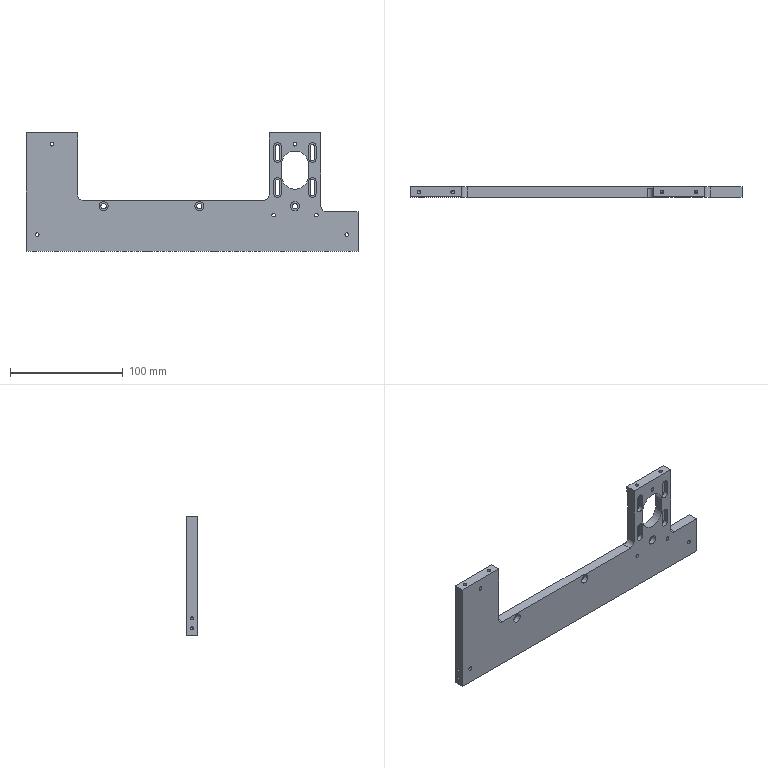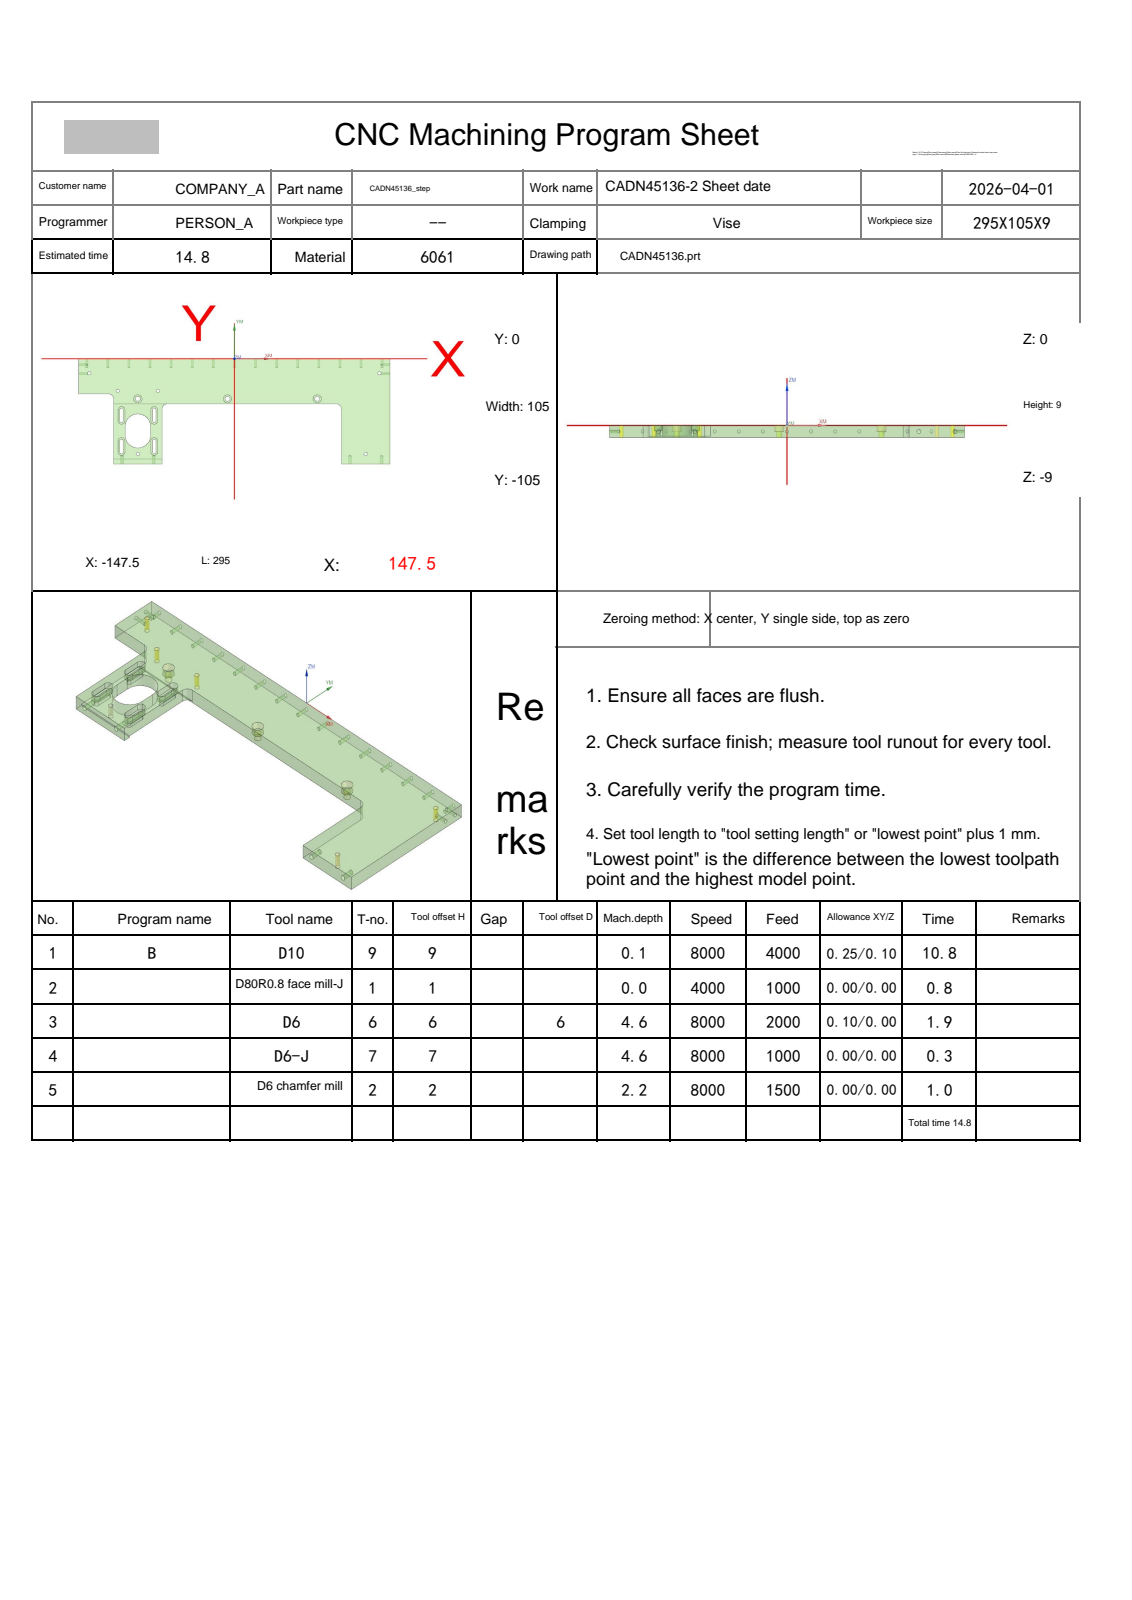NC program | NX | posted by the shop | part box 295 x 9 x 105 mm
Lines 1 to 770 of 3343:
%
O0001
(Machine time: 15.76 MIN)
(===Total Tool:5===)
(T9=D10     D=10.  R=0.   D-  H09 Z=0.1   )
(T1=D80R0.8 face mill-J D=80.  R=0.8  D-  H01 Z=0.    )
(T6=D6      D=6.   R=0.   D6  H06 Z=-4.6  )
(T7=D6-J    D=6.   R=0.   D7  H07 Z=-4.6  )
(T2=D6 chamfer mill   D=6.   R=0.   D-  H02 Z=-2.2  )
G80 G90 G17 G49 G40
G91 G28 Z0
M01
N1 T09 M06
(D10  D=10. R=0. H=09 ce=0.25 di=0.10)
G00 G90 G54 X-1.042 Y13.599 M03 S8000
G43 H09 Z20.
M08
Z2.1
G01 X-1.024 Y13.501 Z1.476 F4000.
X-1.006 Y13.402 Z1.228
X-.988 Y13.304 Z1.046
X-.97 Y13.206 Z.9
X-.952 Y13.107 Z.777
X-.934 Y13.009 Z.672
X-.916 Y12.911 Z.58
X-.898 Y12.812 Z.5
X-.88 Y12.714 Z.43
X-.862 Y12.616 Z.368
X-.844 Y12.517 Z.314
X-.826 Y12.419 Z.267
X-.808 Y12.32 Z.227
X-.79 Y12.222 Z.192
X-.772 Y12.124 Z.164
X-.754 Y12.025 Z.14
X-.737 Y11.927 Z.123
X-.719 Y11.829 Z.11
X-.701 Y11.73 Z.103
X-.683 Y11.632 Z.1
X-.271 Y9.38
G03 X.02 Y9.01 I.503 J.096
X3.263 Y8.4 I3.513 J9.761
X11.624 Y8.192 I8.361 J167.742
X13.491 Y8.202 I0.0 J167.951
G01 X148.128 Y8.183
G02 X154.101 Y4.173 I-.143 J-6.666
X155.462 Y-1.639 I-15.018 J-6.584
X155.704 Y-9.746 I-136.186 J-8.107
X155.695 Y-11.233 I-136.427 J0.0
G01 X155.683 Y-105.63
G02 X151.671 Y-111.602 I-6.664 J.143
X145.703 Y-112.976 I-6.659 J15.278
X136.222 Y-113.219 I-9.481 J184.401
X133.468 Y-113.199 I0.0 J184.644
G01 X-148.17 Y-113.181
G02 X-153.997 Y-109.369 I.158 J6.6
X-155.442 Y-103.579 I14.146 J6.608
X-155.706 Y-95.369 I127.878 J8.21
X-155.695 Y-93.745 I128.141 J0.0
G01 X-155.68 Y.671
G02 X-151.811 Y6.525 I6.619 J-.169
X-145.861 Y7.962 I6.676 J-14.612
X-137.748 Y8.204 I8.112 J-135.802
X-136.266 Y8.196 I0.0 J-136.044
G01 X-2.686 Y8.179
G03 X4.722 Y7.563 I23.47 J237.591
X15.046 Y7.398 I10.324 J322.404
X16.288 Y7.4 I0.0 J322.569
G01 X146.108 Y7.384
G02 X152.709 Y3.222 I-.293 J-7.781
X154.521 Y-3.04 I-14.437 J-7.57
X154.905 Y-11.965 I-103.523 J-8.925
X154.892 Y-13.589 I-103.907 J0.0
G01 X154.879 Y-103.707
G02 X150.784 Y-110.174 I-7.756 J.381
X144.376 Y-112.031 I-7.651 J14.414
X135.464 Y-112.405 I-8.912 J105.999
X133.827 Y-112.392 I0.0 J106.373
G01 X-146.167 Y-112.381
G02 X-152.66 Y-108.304 I.342 J7.752
X-154.529 Y-101.89 I14.346 J7.66
X-154.906 Y-92.925 I106.524 J8.965
X-154.893 Y-91.261 I106.901 J0.0
G01 X-154.881 Y-1.333
G02 X-150.852 Y5.129 I7.744 J-.341
X-144.767 Y6.983 I7.517 J-13.763
X-136.458 Y7.391 I8.309 J-84.332
X-135.421 Y7.385 I0.0 J-84.741
G01 X-4.322 Y7.377
G02 X3.942 Y6.829 I-44.818 J-737.899
G03 X16.194 Y6.592 I12.252 J316.992
X18.528 Y6.601 I0.0 J317.229
G01 X144.268 Y6.579
G02 X151.862 Y1.656 I-.345 J-8.85
X153.721 Y-5.172 I-16.699 J-8.211
X154.102 Y-14.54 I-114.771 J-9.369
X154.091 Y-16.121 I-115.153 J0.0
G01 X154.078 Y-101.781
G02 X149.123 Y-109.38 I-8.847 J.353
X142.283 Y-111.226 I-8.208 J16.824
X133.353 Y-111.594 I-8.931 J108.095
X132.214 Y-111.588 I0.0 J108.463
G01 X-144.326 Y-111.576
G02 X-151.833 Y-106.709 I.392 J8.829
X-153.687 Y-100.123 I16.208 J8.116
X-154.097 Y-90.987 I101.659 J9.136
X-154.088 Y-89.656 I102.068 J0.0
G01 X-154.083 Y-3.356
G02 X-149.226 Y4.322 I8.844 J-.219
X-142.488 Y6.202 I8.189 J-16.333
X-133.467 Y6.595 I9.02 J-103.367
X-132.26 Y6.588 I0.0 J-103.76
G01 X-5.88 Y6.582
G02 X4.55 Y6.018 I-22.742 J-517.372
G03 X18.104 Y5.791 I13.554 J404.888
X20.929 Y5.801 I0.0 J405.115
G01 X142.428 Y5.779
G02 X150.985 Y.337 I-.13 J-9.652
X152.881 Y-6.654 I-17.825 J-8.587
X153.298 Y-16.352 I-112.524 J-9.698
X153.289 Y-17.842 I-112.941 J0.0
G01 X153.278 Y-99.901
G02 X147.729 Y-108.54 I-9.678 J.115
X140.572 Y-110.412 I-8.649 J18.457
X130.965 Y-110.798 I-9.607 J119.204
X129.543 Y-110.79 I0.0 J119.59
G01 X-142.357 Y-110.78
G02 X-151.013 Y-105.281 I.07 J9.672
X-152.897 Y-98.204 I18.157 J8.623
X-153.299 Y-88.521 I116.384 J9.683
X-153.289 Y-87.016 I116.787 J0.0
G01 X-153.279 Y-5.116
G02 X-147.731 Y3.538 I9.686 J-.104
X-140.49 Y5.42 I8.693 J-18.576
X-130.936 Y5.798 I9.553 J-120.599
X-129.54 Y5.79 I0.0 J-120.977
G01 X-6.76 Y5.776
G02 X5.245 Y5.203 I-27.413 J-700.319
G03 X19.831 Y4.991 I14.586 J501.673
X23.008 Y5.001 I0.0 J501.885
G01 X140.748 Y4.978
X140.781
G02 X150.278 Y-1.205 I0.0 J-10.385
X152.099 Y-8.47 I-20.118 J-8.901
X152.494 Y-18.28 I-121.393 J-9.81
X152.487 Y-19.579 I-121.789 J0.0
G01 X152.477 Y-98.199
X152.478 Y-98.282
G02 X146.307 Y-107.772 I-10.383 J0.0
X138.891 Y-109.614 I-8.969 J20.269
X129.14 Y-109.994 I-9.751 J124.677
X127.861 Y-109.988 I0.0 J125.057
G01 X-140.758 Y-109.975
X-140.792
G02 X-150.243 Y-103.866 I0.0 J10.365
X-152.115 Y-96.374 I20.166 J9.018
X-152.494 Y-86.658 I124.333 J9.716
X-152.488 Y-85.424 I124.712 J0.0
G01 X-152.474 Y-6.724
Y-6.712
G02 X-146.318 Y2.767 I10.375 J0.0
X-139.141 Y4.587 I8.872 J-19.921
X-129.221 Y4.996 I9.92 J-119.985
X-127.792 Y4.988 I0.0 J-120.395
G01 X-7.652 Y4.975
G02 X5.16 Y4.417 I-21.37 J-638.689
G03 X20.407 Y4.192 I15.247 J516.842
X23.488 Y4.202 I0.0 J517.067
G01 X139.148 Y4.177
X139.271 Y4.178
G02 X145.984 Y1.999 I0.0 J-11.431
X150.263 Y-4.534 I-8.054 J-9.944
X151.499 Y-12.66 I-32.537 J-9.105
X151.719 Y-25.287 I-362.488 J-12.627
X151.698 Y-29.217 I-362.708 J0.0
G01 X151.677 Y-96.557
X151.679 Y-96.726
G02 X149.706 Y-103.204 I-11.62 J0.0
X143.206 Y-107.687 I-10.008 J7.557
X135.249 Y-108.976 I-9.062 J30.727
X124.188 Y-109.209 I-11.061 J262.82
X121.653 Y-109.197 I0.0 J263.052
G01 X-139.127 Y-109.175
X-139.258 Y-109.176
G02 X-145.952 Y-107.022 I0.0 J11.48
X-150.277 Y-100.42 I8.041 J9.985
X-151.506 Y-92.212 I32.969 J9.136
X-151.718 Y-79.639 I373.131 J12.573
X-151.698 Y-75.735 I373.343 J0.0
G01 X-151.673 Y-8.315
Y-8.213
G02 X-149.486 Y-1.503 I11.387 J0.0
X-142.871 Y2.792 I9.977 J-8.126
X-134.74 Y4.005 I9.092 J-33.074
X-122.127 Y4.219 I12.613 J-371.929
X-118.182 Y4.198 I0.0 J-372.143
G01 X-8.522 Y4.174
G02 X5.864 Y3.601 I-23.554 J-772.256
G03 X21.43 Y3.394 I15.566 J585.251
X24.368 Y3.402 I0.0 J585.458
G01 X137.468 Y3.382
G02 X137.692 Y3.384 I.224 J-13.158
X143.714 Y1.926 I0.0 J-13.16
X149.031 Y-4.551 I-6.152 J-10.472
X150.617 Y-12.853 I-27.515 J-9.559
X150.914 Y-24.635 I-233.501 J-11.782
X150.896 Y-27.568 I-233.798 J0.0
G01 X150.878 Y-94.988
G02 X150.88 Y-95.199 I-13.158 J-.211
X149.452 Y-101.161 I-13.159 J0.0
X143.124 Y-106.463 I-10.434 J6.026
X135.236 Y-108.073 I-9.392 J25.881
X124.51 Y-108.403 I-10.725 J174.014
X122.603 Y-108.393 I0.0 J174.344
G01 X-137.537 Y-108.377
X-137.735 Y-108.378
G02 X-143.913 Y-106.81 I0.0 J12.949
X-149.074 Y-100.334 I6.443 J10.429
X-150.615 Y-92.187 I27.721 J9.461
X-150.915 Y-80.371 I232.213 J11.816
X-150.896 Y-77.392 I232.513 J0.0
G01 X-150.877 Y-9.972
X-150.878 Y-9.775
G02 X-149.352 Y-3.662 I13. J0.0
X-143.008 Y1.506 I10.402 J-6.291
X-134.874 Y3.101 I9.476 J-26.788
X-124.315 Y3.401 I10.559 J-185.945
X-122.56 Y3.392 I0.0 J-186.244
G01 X-9.38 Y3.375
G02 X5.387 Y2.825 I-16.941 J-653.015
G03 X22.135 Y2.593 I16.748 J603.489
X25.488 Y2.602 I0.0 J603.721
G01 X136.188 Y2.577
X136.37 Y2.579
G02 X142.462 Y1.185 I0.0 J-14.012
X148.057 Y-5.299 I-5.926 J-10.769
X149.766 Y-13.571 I-26.358 J-9.757
X150.109 Y-25.105 I-193.559 J-11.534
X150.094 Y-27.564 I-193.902 J0.0
G01 X150.079 Y-93.464
G02 X150.082 Y-93.753 I-14.601 J-.289
X148.823 Y-99.686 I-14.604 J0.0
X142.273 Y-105.528 I-10.848 J5.57
X134.325 Y-107.233 I-9.618 J25.454
X123.377 Y-107.601 I-10.948 J162.529
X121.533 Y-107.591 I0.0 J162.898
G01 X-135.967 Y-107.579
G02 X-136.251 Y-107.582 I-.285 J14.603
X-142.189 Y-106.321 I0.0 J14.605
X-148.007 Y-99.82 I5.558 J10.827
X-149.756 Y-91.556 I25.794 J9.774
X-150.099 Y-80.759 I169.356 J10.797
X-150.09 Y-79.004 I169.7 J0.0
G01 X-150.074 Y-11.344
G02 X-150.076 Y-11.137 I14.003 J.207
X-148.625 Y-4.929 I14.004 J0.0
X-142.165 Y.57 I10.742 J-6.074
X-134.046 Y2.256 I9.668 J-26.161
X-122.365 Y2.611 I11.681 J-192.34
X-119.813 Y2.594 I0.0 J-192.695
G01 X-10.233 Y2.577
G02 X6.173 Y2.006 I-18.598 J-770.274
G03 X22.893 Y1.796 I16.72 J665.43
X25.888 Y1.802 I0.0 J665.64
G01 X134.588 Y1.783
G02 X134.896 Y1.786 I.308 J-15.827
X140.912 Y.598 I0.0 J-15.83
X147.098 Y-6.055 I-5.326 J-11.154
X148.894 Y-14.065 I-25.062 J-9.825
X149.298 Y-25.195 I-153.026 J-11.13
X149.289 Y-26.934 I-153.43 J0.0
G01 X149.276 Y-92.194
G02 X149.278 Y-92.466 I-15.489 J-.271
X148.051 Y-98.508 I-15.491 J0.0
X141.479 Y-104.583 I-11.107 J5.424
X133.155 Y-106.42 I-9.985 J25.465
X121.693 Y-106.805 I-11.462 J170.608
X119.564 Y-106.791 I0.0 J170.992
G01 X-134.736 Y-106.775
G02 X-134.974 Y-106.777 I-.239 J15.483
X-140.982 Y-105.564 I0.0 J15.484
X-147.132 Y-98.864 I5.426 J11.153
X-148.903 Y-90.843 I25.455 J9.827
X-149.299 Y-79.739 I155.791 J11.104
X-149.289 Y-77.972 I156.186 J0.0
G01 X-149.271 Y-12.633
X-149.272 Y-12.451
G02 X-147.976 Y-6.335 I15.078 J0.0
X-141.234 Y-.315 I11.137 J-5.687
X-132.81 Y1.45 I9.979 J-26.643
X-121.588 Y1.802 I11.222 J-178.732
X-119.618 Y1.791 I0.0 J-179.084
G01 X-11.158 Y1.779
G02 X5.854 Y1.221 I-14.287 J-695.118
G03 X22.663 Y1. I16.809 J638.744
X24.689 Y1.003 I0.0 J638.965
G01 X133.388 Y.98
G02 X133.653 Y.982 I.265 J-16.768
X139.651 Y-.128 I0.0 J-16.77
X146.18 Y-6.878 I-5.078 J-11.443
X148.09 Y-15.268 I-25.295 J-10.171
X148.502 Y-26.848 I-162.533 J-11.581
X148.489 Y-28.858 I-162.946 J0.0
G01 X148.472 Y-90.997
G02 X148.474 Y-91.236 I-16.272 J-.238
X147.26 Y-97.402 I-16.274 J0.0
X140.574 Y-103.699 I-11.368 J5.371
X132.336 Y-105.58 I-10.09 J25.217
X121.468 Y-105.99 I-10.867 J143.791
X120.186 Y-105.984 I0.0 J144.201
G01 X-133.474 Y-105.973
G02 X-133.725 Y-105.974 I-.251 J16.335
X-139.877 Y-104.772 I0.0 J16.337
X-146.157 Y-98.172 I5.319 J11.349
X-148.062 Y-90.024 I24.703 J10.071
X-148.491 Y-79.056 I139.98 J10.968
X-148.484 Y-77.715 I140.409 J0.0
G01 X-148.473 Y-14.056
G02 X-148.475 Y-13.804 I16.505 J.251
X-147.314 Y-7.724 I16.507 J0.0
X-140.649 Y-1.334 I11.387 J-5.208
X-132.343 Y.579 I10.135 J-25.013
X-121.513 Y.989 I10.829 J-142.782
X-120.273 Y.984 I0.0 J-143.192
G01 X-11.173 Y.972
G02 X6.881 Y.395 I-21.697 J-962.456
G03 X23.793 Y.2 I16.912 J730.973
X25.969 Y.203 I0.0 J731.169
G01 X132.028 Y.182
G02 X132.357 Y.185 I.329 J-18.071
X138.464 Y-.878 I0.0 J-18.074
X145.286 Y-7.734 I-4.904 J-11.7
X147.262 Y-16.192 I-25.181 J-10.344
X147.701 Y-27.987 I-158.212 J-11.794
X147.688 Y-30.021 I-158.651 J0.0
G01 X147.672 Y-89.681
G02 X147.674 Y-89.962 I-17.445 J-.281
X146.529 Y-96.18 I-17.447 J0.0
X139.81 Y-102.765 I-11.615 J5.131
X131.754 Y-104.717 I-10.17 J24.374
X120.47 Y-105.19 I-11.284 J134.156
X119.048 Y-105.183 I0.0 J134.63
G01 X-132.212 Y-105.172
G02 X-132.475 Y-105.174 I-.263 J17.377
X-138.709 Y-104.017 I0.0 J17.379
X-145.341 Y-97.139 I5.196 J11.647
X-147.276 Y-88.669 I25.668 J10.318
X-147.702 Y-76.836 I163.921 J11.832
X-147.689 Y-74.759 I164.347 J0.0
G01 X-147.673 Y-15.339
G02 X-147.675 Y-15.055 I17.541 J.284
X-146.536 Y-8.838 I17.543 J0.0
X-139.664 Y-2.171 I11.662 J-5.146
X-131.438 Y-.251 I10.223 J-25.219
X-120.35 Y.188 I11.087 J-139.656
X-119.05 Y.182 I0.0 J-140.096
G01 X-12.03 Y.174
G02 X6.245 Y-.382 I-15.656 J-814.736
G03 X23.967 Y-.6 I17.722 J718.369
X26.289 Y-.597 I0.0 J718.587
G01 X130.748 Y-.618
G02 X131.097 Y-.615 I.348 J-19.457
X137.203 Y-1.598 I0.0 J-19.46
X144.348 Y-8.47 I-4.602 J-11.933
X146.408 Y-16.829 I-24.414 J-10.451
X146.885 Y-28.059 I-131.929 J-11.23
X146.879 Y-29.295 I-132.406 J0.0
G01 X146.875 Y-88.315
G02 X146.878 Y-88.657 I-19.049 J-.342
X145.846 Y-94.84 I-19.052 J0.0
X138.847 Y-101.929 I-11.926 J4.775
X130.633 Y-103.912 I-10.35 J24.864
X119.202 Y-104.39 I-11.431 J136.647
X117.767 Y-104.382 I0.0 J137.125
G01 X-130.853 Y-104.374
G02 X-131.167 Y-104.377 I-.314 J19.039
X-137.301 Y-103.361 I0.0 J19.042
X-144.41 Y-96.392 I4.731 J11.936
X-146.423 Y-88.028 I24.936 J10.426
X-146.888 Y-76.687 I137.999 J11.341
X-146.882 Y-75.321 I138.464 J0.0
G01 X-146.875 Y-16.701
G02 X-146.878 Y-16.368 I19.259 J.333
X-145.88 Y-10.25 I19.262 J0.0
X-138.893 Y-3.092 I11.947 J-4.672
X-130.764 Y-1.103 I10.314 J-24.541
X-119.319 Y-.612 I11.445 J-133.096
X-117.898 Y-.619 I0.0 J-133.587
G01 X-12.878 Y-.624
G02 X6.085 Y-1.173 I-13.148 J-780.897
G03 X24.808 Y-1.403 I18.723 J763.395
X27.889 Y-1.397 I0.0 J763.625
G01 X129.708 Y-1.422
G02 X130.007 Y-1.419 I.298 J-19.874
X136.24 Y-2.422 I0.0 J-19.876
X143.541 Y-9.474 I-4.665 J-12.135
X145.603 Y-17.914 I-24.987 J-10.575
X146.084 Y-29.282 I-134.004 J-11.368
X146.079 Y-30.46 I-134.485 J0.0
G01 X146.074 Y-87.08
G02 X146.077 Y-87.434 I-20.386 J-.354
X145.117 Y-93.62 I-20.389 J0.0
X138.173 Y-100.971 I-12.128 J4.501
X129.754 Y-103.085 I-10.592 J24.363
X118.099 Y-103.589 I-11.655 J134.466
X116.649 Y-103.581 I0.0 J134.971
G01 X-129.731 Y-103.571
G02 X-130.037 Y-103.574 I-.306 J19.668
X-136.337 Y-102.538 I0.0 J19.67
X-143.588 Y-95.42 I4.798 J12.14
X-145.63 Y-86.816 I25.615 J10.625
X-146.086 Y-75.438 I141.783 J11.378
X-146.081 Y-74.188 I142.239 J0.0
G01 X-146.074 Y-17.888
G02 X-146.076 Y-17.563 I20.449 J.325
X-145.133 Y-11.425 I20.452 J0.0
X-138.05 Y-3.972 I12.182 J-4.486
X-129.535 Y-1.892 I10.609 J-24.965
X-118.038 Y-1.413 I11.497 J-137.63
X-116.668 Y-1.42 I0.0 J-138.109
G01 X-12.848 Y-1.429
G02 X6.717 Y-1.988 I-16.701 J-927.382
G03 X25.212 Y-2.202 I18.496 J797.81
X28.289 Y-2.196 I0.0 J798.024
G01 X128.108 Y-2.214
G02 X128.579 Y-2.209 I.47 J-22.807
X134.75 Y-3.059 I0.0 J-22.812
X142.62 Y-10.214 I-4.101 J-12.418
X144.778 Y-18.789 I-24.668 J-10.765
X145.284 Y-30.396 I-132.82 J-11.607
X145.278 Y-31.654 I-133.326 J0.0
G01 X145.279 Y-85.634
G02 X145.284 Y-86.096 I-22.726 J-.462
X144.428 Y-92.274 I-22.731 J0.0
X137.082 Y-100.213 I-12.469 J4.169
X128.491 Y-102.301 I-10.72 J25.386
X116.831 Y-102.787 I-11.66 J139.7
X115.465 Y-102.78 I0.0 J140.186
G01 X-128.195 Y-102.778
G02 X-128.635 Y-102.782 I-.44 J22.458
X-134.832 Y-101.91 I0.0 J22.463
X-142.567 Y-94.895 I4.168 J12.367
X-144.737 Y-86.57 I23.91 J10.679
X-145.28 Y-75.018 I122.634 J11.553
X-145.275 Y-73.868 I123.177 J0.0
G01 X-145.279 Y-19.408
G02 X-145.284 Y-18.95 I23.289 J.458
X-144.489 Y-12.918 I23.293 J0.0
X-137.252 Y-4.865 I12.466 J-3.925
X-128.831 Y-2.736 I10.685 J-24.542
X-117.395 Y-2.221 I11.436 J-126.686
X-116.367 Y-2.225 I0.0 J-127.201
G01 X-13.507 Y-2.228
G02 X6.953 Y-2.791 I-15.92 J-950.714
G03 X25.301 Y-3.001 I18.348 J800.206
X28.289 Y-2.996 I0.0 J800.416
G01 X127.309 Y-3.02
G02 X127.645 Y-3.018 I.336 J-22.38
X133.941 Y-3.922 I0.0 J-22.382
X141.858 Y-11.279 I-4.313 J-12.579
X143.969 Y-19.79 I-25.303 J-10.791
X144.484 Y-31.582 I-134.68 J-11.792
X144.478 Y-32.895 I-135.195 J0.0
G01 X144.474 Y-84.715
G02 X144.477 Y-85.112 I-22.579 J-.397
X143.576 Y-91.429 I-22.582 J0.0
X136.33 Y-99.306 I-12.56 J4.284
X127.67 Y-101.473 I-10.878 J25.079
X115.643 Y-101.989 I-12.027 J139.765
X114.085 Y-101.981 I0.0 J140.281
G01 X-127.015 Y-101.978
G02 X-127.483 Y-101.982 I-.468 J23.641
X-133.738 Y-101.14 I0.0 J23.645
X-141.795 Y-93.853 I4.078 J12.605
X-143.943 Y-85.436 I24.626 J10.769
X-144.481 Y-73.721 I127.363 J11.715
X-144.475 Y-72.492 I127.901 J0.0
G01 X-144.478 Y-20.513
G02 X-144.482 Y-20.07 I24.308 J.442
X-143.716 Y-14.018 I24.312 J0.0
X-136.256 Y-5.66 I12.7 J-3.827
X-127.674 Y-3.528 I10.832 J-25.269
X-115.667 Y-3.011 I12.008 J-139.276
X-114.089 Y-3.02 I0.0 J-139.792
G01 X-14.349 Y-3.026
G02 X7.031 Y-3.59 I-14.475 J-953.625
G03 X25.408 Y-3.801 I18.377 J802.198
X28.289 Y-3.795 I0.0 J802.408
G01 X125.948 Y-3.816
G02 X126.362 Y-3.812 I.414 J-24.772
X132.6 Y-4.61 I0.0 J-24.775
X140.999 Y-12.12 I-3.91 J-12.826
X143.161 Y-20.782 I-25.409 J-10.943
X143.683 Y-32.699 I-135.681 J-11.917
X143.677 Y-34.046 I-136.204 J0.0
G01 Y-83.386
G02 X143.682 Y-83.862 I-24.664 J-.475
X142.855 Y-90.194 I-24.668 J0.0
X135.55 Y-98.416 I-12.758 J3.979
X127.145 Y-100.612 I-10.872 J24.432
X115.544 Y-101.173 I-11.601 J119.755
X114.683 Y-101.17 I0.0 J120.316
G01 X-126.097 Y-101.173
G02 X-126.5 Y-101.177 I-.404 J23.594
X-132.895 Y-100.294 I0.0 J23.598
X-140.965 Y-92.95 I4.204 J12.725
X-143.152 Y-84.299 I25.129 J10.956
X-143.681 Y-72.444 I132.454 J11.855
X-143.676 Y-71.195 I132.984 J0.0
G01 X-143.677 Y-21.615
G02 X-143.681 Y-21.151 I24.852 J.465
X-142.878 Y-14.885 I24.856 J0.0
X-135.501 Y-6.56 I12.789 J-3.903
X-126.77 Y-4.345 I11.014 J-25.104
X-114.915 Y-3.818 I11.855 J-133.123
X-113.666 Y-3.824 I0.0 J-133.65
G01 X-14.166 Y-3.832
G02 X5.919 Y-4.358 I-12.502 J-860.779
G03 X25.822 Y-4.6 I19.903 J816.047
X28.769 Y-4.595 I0.0 J816.29
G01 X124.908 Y-4.617
G02 X125.327 Y-4.613 I.419 J-25.141
X131.719 Y-5.439 I0.0 J-25.145
X140.174 Y-13.022 I-3.991 J-12.956
X142.327 Y-21.522 I-25.352 J-10.946
X142.877 Y-33.402 I-127.98 J-11.879
X142.872 Y-34.545 I-128.53 J0.0
G01 Y-82.525
G02 X142.875 Y-82.921 I-24.44 J-.396
X142.021 Y-89.328 I-24.444 J0.0
X134.48 Y-97.67 I-12.922 J4.101
X125.828 Y-99.844 I-11.018 J25.551
X113.68 Y-100.385 I-12.148 J136.088
X112.245 Y-100.377 I0.0 J136.629
G01 X-125.015 Y-100.373
G02 X-125.381 Y-100.375 I-.366 J24.966
X-131.666 Y-99.571 I0.0 J24.968
X-140.081 Y-92.171 I3.898 J12.917
X-142.32 Y-83.535 I24.826 J11.046
X-142.873 Y-71.817 I123.934 J11.718
X-142.87 Y-70.912 I124.487 J0.0
G01 X-142.871 Y-22.453
G02 X-142.874 Y-22.08 I24.528 J.373
X-142.037 Y-15.727 I24.531 J0.0
X-134.502 Y-7.339 I12.915 J-4.024
X-125.926 Y-5.167 I10.989 J-25.372
X-114.253 Y-4.627 I11.673 J-125.838
X-113.383 Y-4.63 I0.0 J-126.378
G01 X-14.843
G02 X5.838 Y-5.153 I-11.424 J-861.077
G03 X26.521 Y-5.404 I20.683 J852.762
X30.369 Y-5.395 I0.0 J853.013
G01 X123.788 Y-5.416
G02 X124.218 Y-5.413 I.429 J-26.441
X130.604 Y-6.195 I0.0 J-26.444
X139.229 Y-13.66 I-3.77 J-13.071
X141.468 Y-22.05 I-24.439 J-11.017
X142.071 Y-34.006 I-118.313 J-11.956
X142.067 Y-34.989 I-118.916 J0.0
G01 X142.072 Y-81.449
G02 X142.075 Y-81.854 I-25.265 J-.404
X141.229 Y-88.335 I-25.269 J0.0
X133.626 Y-96.827 I-13.068 J4.051
X124.898 Y-99.033 I-11.124 J25.644
X112.97 Y-99.577 I-11.928 J130.613
X111.875 Y-99.572 I0.0 J131.157
G01 X-123.945
G02 X-124.342 Y-99.575 I-.397 J25.474
X-130.756 Y-98.754 I0.0 J25.477
X-139.34 Y-91.103 I3.961 J13.085
X-141.545 Y-82.292 I25.872 J11.157
X-142.076 Y-70.413 I132.527 J11.879
X-142.072 Y-69.349 I133.058 J0.0
G01 X-142.071 Y-23.529
G02 X-142.074 Y-23.153 I25.417 J.376
X-141.246 Y-16.72 I25.42 J0.0
X-133.648 Y-8.181 I13.061 J-3.972
X-124.84 Y-5.96 I11.165 J-25.708
X-112.89 Y-5.422 I11.95 J-132.416
X-111.736 Y-5.427 I0.0 J-132.955
G01 X-15.436 Y-5.43
G02 X6.552 Y-5.97 I-11.863 J-929.752
G03 X26.132 Y-6.201 I19.581 J832.078
X29.329 Y-6.194 I0.0 J832.309
G01 X122.908 Y-6.22
G02 X123.307 Y-6.217 I.399 J-25.953
X129.875 Y-7.061 I0.0 J-25.956
X138.449 Y-14.636 I-3.99 J-13.157
X140.694 Y-23.269 I-25.228 J-11.168
X141.272 Y-35.277 I-124.467 J-12.008
X141.268 Y-36.29 I-125.045 J0.0
G01 X141.272 Y-80.35
G02 X141.275 Y-80.761 I-26.502 J-.411
X140.47 Y-87.243 I-26.505 J0.0
X132.865 Y-95.945 I-13.212 J3.872
X124.148 Y-98.204 I-11.207 J25.301
X112.373 Y-98.768 I-11.775 J122.511
X111.606 Y-98.766 I0.0 J123.076
G01 X100.726 Y-98.793
X-122.853 Y-98.772
G02 X-123.288 Y-98.775 I-.435 J26.143
X-129.9 Y-97.926 I0.0 J26.147
X-138.436 Y-90.387 I4.02 J13.153
X-140.709 Y-81.598 I25.341 J11.244
X-141.271 Y-69.705 I125.738 J11.893
X-141.268 Y-68.816 I126.299 J0.0
G01 X-141.272 Y-24.676
G02 X-141.275 Y-24.243 I26.482 J.433
X-140.456 Y-17.705 I26.485 J0.0
X-132.863 Y-9.051 I13.175 J-3.902
X-124.227 Y-6.806 I11.183 J-25.275
X-112.255 Y-6.229 I11.973 J-123.959
X-111.286 Y-6.233 I0.0 J-124.536
G01 X-16.186 Y-6.228
G02 X7.107 Y-6.782 I-11.722 J-981.444
G03 X26.36 Y-7.002 I19.254 J845.613
X29.889 Y-6.994 I0.0 J845.832
G01 X121.868 Y-7.02
G02 X122.239 Y-7.017 I.371 J-27.189
X128.763 Y-7.811 I0.0 J-27.191
X137.697 Y-15.663 I-3.839 J-13.376
X139.901 Y-24.318 I-25.959 J-11.218
X140.474 Y-36.52 I-129.534 J-12.203
X140.469 Y-37.659 I-130.108 J0.0
G01 X140.471 Y-79.319
G02 X140.474 Y-79.755 I-26.91 J-.436
X139.649 Y-86.37 I-26.913 J0.0
X131.886 Y-95.171 I-13.334 J3.937
X123.007 Y-97.42 I-11.325 J26.05
X110.945 Y-97.974 I-12.062 J131.117
X109.904 Y-97.97 I0.0 J131.671
G01 X-121.516 Y-97.976
G02 X-122.032 Y-97.98 I-.516 J29.119
X-128.501 Y-97.253 I0.0 J29.123
X-137.66 Y-89.41 I3.553 J13.418
X-139.909 Y-80.613 I25.805 J11.282
X-140.473 Y-68.506 I129.51 J12.107
X-140.469 Y-67.431 I130.075 J0.0
G01 X-140.47 Y-25.691
G02 X-140.473 Y-25.292 I27.542 J.399
X-139.696 Y-18.794 I27.545 J0.0
X-132.03 Y-9.897 I13.325 J-3.731
X-123.32 Y-7.616 I11.272 J-25.274
X-111.06 Y-7.025 I12.26 J-126.963
X-109.9 Y-7.031 I0.0 J-127.554
G01 X-16.8 Y-7.027
G02 X5.993 Y-7.552 I-9.441 J-904.634
G03 X26.766 Y-7.802 I20.773 J862.378
X30.529 Y-7.794 I0.0 J862.628
G01 X120.908 Y-7.821
G02 X121.28 Y-7.818 I.372 J-27.272
X127.959 Y-8.649 I0.0 J-27.275
X136.765 Y-16.301 I-3.914 J-13.397
X139.075 Y-25.087 I-25.357 J-11.366
X139.669 Y-37.252 I-124.378 J-12.165
X139.665 Y-38.187 I-124.972 J0.0
G01 X139.675 Y-78.007
G02 X139.68 Y-78.542 I-29.42 J-.535
X138.928 Y-85.149 I-29.425 J0.0
X131.124 Y-94.297 I-13.499 J3.614
X122.57 Y-96.556 I-11.259 J25.309
X110.375 Y-97.169 I-12.195 J121.056
X109.391 Y-97.165 I0.0 J121.669
G01 X97.951 Y-97.192
X-120.909 Y-97.168
G02 X-121.295 Y-97.171 I-.386 J27.245
X-127.96 Y-96.343 I0.0 J27.248
X-136.81 Y-88.6 I3.929 J13.419
X-139.059 Y-80.043 I25.365 J11.243
X-139.669 Y-67.812 I122.332 J12.231
X-139.665 Y-66.784 I122.942 J0.0
G01 X-139.674 Y-26.964
G02 X-139.678 Y-26.465 I29.632 J.498
X-138.942 Y-19.899 I29.636 J0.0
X-131.099 Y-10.69 I13.504 J-3.556
X-122.307 Y-8.412 I11.354 J-25.725
X-110.248 Y-7.832 I12.059 J-124.947
X-109.366 Y-7.835 I0.0 J-125.527
G01 X-20.026 Y-7.815
G02 X5.912 Y-8.348 I-5.08 J-878.077
G03 X26.818 Y-8.601 I20.906 J863.203
X30.449 Y-8.594 I0.0 J863.456
G01 X119.868 Y-8.62
G02 X120.245 Y-8.618 I.376 J-28.268
X126.924 Y-9.418 I0.0 J-28.271
X135.992 Y-17.269 I-3.807 J-13.561
X138.257 Y-25.9 I-25.613 J-11.333
X138.857 Y-37.771 I-116.979 J-11.871
X138.856 Y-38.279 I-117.579 J0.0
G01 X138.892 Y-51.079
X138.868 Y-77.379
G02 X138.871 Y-77.783 I-27.915 J-.404
X138.048 Y-84.511 I-27.918 J0.0
X130.096 Y-93.553 I-13.562 J3.91
X121.291 Y-95.793 I-11.387 J26.335
X108.975 Y-96.373 I-12.317 J130.63
X107.87 Y-96.368 I0.0 J131.209
G01 X-119.79 Y-96.37
G02 X-120.206 Y-96.373 I-.415 J28.733
X-126.849 Y-95.594 I0.0 J28.736
X-136.044 Y-87.619 I3.742 J13.602
X-138.29 Y-78.813 I26.264 J11.391
X-138.872 Y-66.486 I130.319 J12.327
X-138.868 Y-65.391 I130.9 J0.0
G01 X-138.869 Y-27.731
G02 X-138.873 Y-27.293 I28.644 J.438
X-138.079 Y-20.594 I28.648 J0.0
X-130.169 Y-11.481 I13.565 J-3.783
X-121.534 Y-9.236 I11.321 J-25.819
X-109.113 Y-8.628 I12.421 J-126.635
X-108.034 Y-8.633 I0.0 J-127.242
G01 X-17.094 Y-8.631
G02 X6.627 Y-9.165 I-9.622 J-955.431
G03 X27.102 Y-9.403 I20.475 J880.216
X31.169 Y-9.394 I0.0 J880.455
G01 X118.428 Y-9.413
G02 X118.947 Y-9.409 I.518 J-31.903
X125.579 Y-10.106 I0.0 J-31.907
X135.168 Y-18.12 I-3.367 J-13.773
X137.481 Y-27.066 I-26.087 J-11.518
X138.066 Y-39.239 I-126.458 J-12.173
X138.063 Y-40.087 I-127.043 J0.0
G01 X138.074 Y-75.986
G02 X138.079 Y-76.539 I-30.788 J-.553
X137.33 Y-83.29 I-30.793 J0.0
X129.332 Y-92.688 I-13.708 J3.564
X120.374 Y-94.988 I-11.519 J26.268
X108.169 Y-95.568 I-12.205 J128.253
X107.273 Y-95.564 I0.0 J128.832
G01 X97.593 Y-95.591
X-118.787 Y-95.569
G02 X-119.195 Y-95.572 I-.407 J29.66
X-125.849 Y-94.816 I0.0 J29.663
X-135.212 Y-86.782 I3.635 J13.709
X-137.494 Y-77.825 I26.458 J11.509
X-138.075 Y-65.261 I135.475 J12.564
X-138.069 Y-64.003 I136.056 J0.0
G01 X-138.068 Y-28.663
G02 X-138.071 Y-28.239 I28.845 J.424
X-137.26 Y-21.448 I28.848 J0.0
X-129.373 Y-12.331 I13.629 J-3.82
X-120.426 Y-10.018 I11.514 J-26.078
X-108.311 Y-9.436 I12.115 J-125.758
X-107.565 Y-9.438 I0.0 J-126.34
G01 X-25.585 Y-9.409
G02 X7.262 Y-9.979 I-.768 J-991.587
G03 X28.121 Y-10.21 I20.859 J940.717
X33.648 Y-10.194 I0.0 J940.948
G01 X117.788 Y-10.219
G02 X118.19 Y-10.216 I.402 J-30.365
X124.931 Y-10.974 I0.0 J-30.367
X134.409 Y-19.103 I-3.628 J-13.82
X136.695 Y-28.139 I-26.777 J-11.583
X137.27 Y-40.525 I-133.22 J-12.386
X137.266 Y-41.561 I-133.794 J0.0
G01 X137.268 Y-75.301
G02 X137.272 Y-75.752 I-29.668 J-.451
X136.471 Y-82.598 I-29.672 J0.0
X128.447 Y-91.882 I-13.75 J3.774
X119.649 Y-94.162 I-11.49 J26.233
X107.462 Y-94.762 I-12.187 J123.287
X106.709 Y-94.76 I0.0 J123.888
G01 X94.389 Y-94.791
X-117.75 Y-94.769
G02 X-118.223 Y-94.773 I-.472 J29.952
X-125.049 Y-93.985 I0.0 J29.956
X-134.407 Y-85.898 I3.736 J13.78
X-136.677 Y-77.022 I26.51 J11.508
X-137.271 Y-64.495 I131.657 J12.527